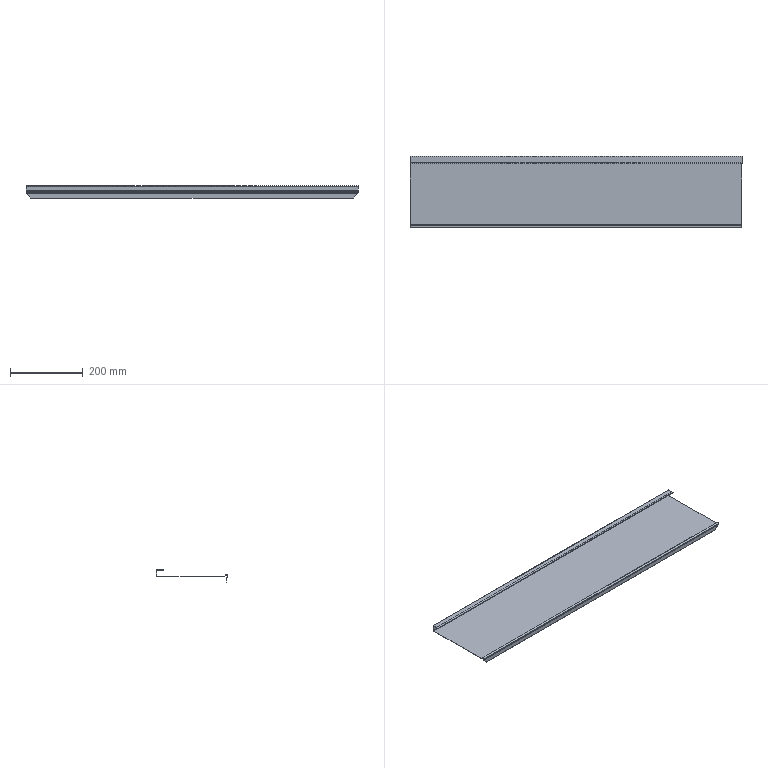Part | SolidWorks | features SM3dBend 4, EdgeFlange 2, FlatPattern 1, Hem 1, SMBaseFlange 1, SheetMetal 1 | 1 solid | 64 faces | box 915 x 196.571 x 33.2 mm | volume 189594 mm3 | plane 48 | cylinder 14 | spline 2 | commonest cylinder face diameters 1 x3 2.6 x3 0.1 x1 1.2 x1 1.7 x1 2.8 x1